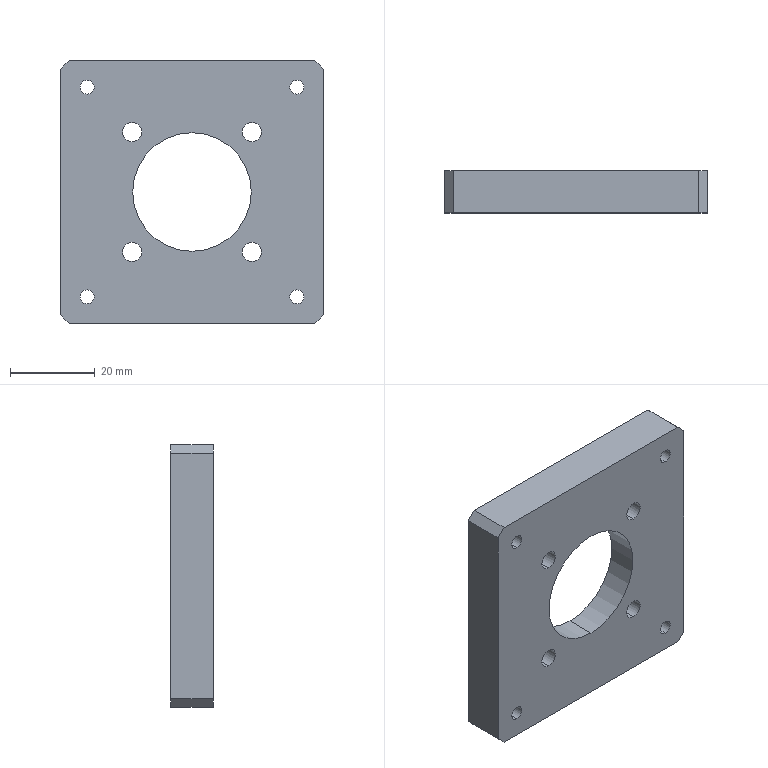Part | STEP file | KK60-F2E KK60 200W flange | 1 solid | 43 faces | box 62 x 10 x 62 mm | volume 27303 mm3 | cylinder 28 | plane 15 | commonest cylinder face diameters 3.3 x8 4.5 x8 8 x8 28 x2 50 x2